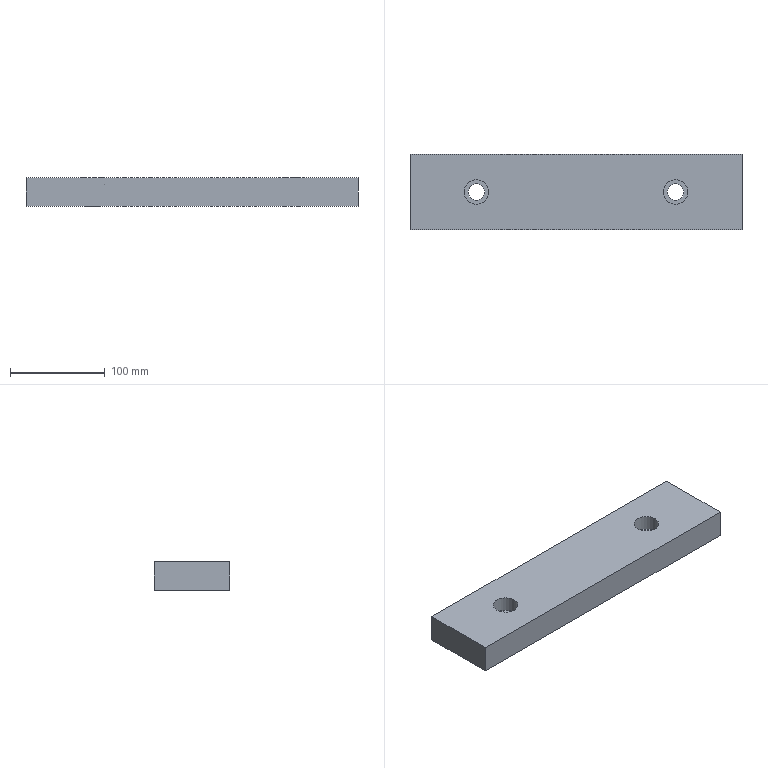Part | NX | features clamp plate 2 | 1 solid | 12 faces | box 350 x 80 x 30 mm | volume 816275 mm3 | plane 8 | cylinder 4 | commonest cylinder face diameters 17.5 x2 26 x2
STEP:
#1=CARTESIAN_POINT('',(-92.,0.,30.));
#2=VERTEX_POINT('',#1);
#3=CARTESIAN_POINT('',(-105.,0.,30.));
#4=DIRECTION('',(0.,0.,1.));
#5=DIRECTION('',(1.,0.,0.));
#6=AXIS2_PLACEMENT_3D('',#3,#4,#5);
#7=CIRCLE('',#6,13.);
#8=EDGE_CURVE('',#2,#2,#7,.F.);
#9=ORIENTED_EDGE('',*,*,#8,.F.);
#10=EDGE_LOOP('',(#9));
#11=FACE_BOUND('',#10,.T.);
#12=CARTESIAN_POINT('',(-92.,0.,14.));
#13=VERTEX_POINT('',#12);
#14=CARTESIAN_POINT('',(-105.,0.,14.));
#15=DIRECTION('',(0.,0.,1.));
#16=DIRECTION('',(1.,0.,0.));
#17=AXIS2_PLACEMENT_3D('',#14,#15,#16);
#18=CIRCLE('',#17,13.);
#19=EDGE_CURVE('',#13,#13,#18,.F.);
#20=ORIENTED_EDGE('',*,*,#19,.T.);
#21=EDGE_LOOP('',(#20));
#22=FACE_BOUND('',#21,.T.);
#23=CARTESIAN_POINT('',(-105.,0.,30.));
#24=DIRECTION('',(0.,0.,1.));
#25=DIRECTION('',(1.,0.,0.));
#26=AXIS2_PLACEMENT_3D('',#23,#24,#25);
#27=CYLINDRICAL_SURFACE('',#26,13.);
#28=ADVANCED_FACE('',(#11,#22),#27,.F.);
#29=CARTESIAN_POINT('',(118.,0.,30.));
#30=VERTEX_POINT('',#29);
#31=CARTESIAN_POINT('',(105.,0.,30.));
#32=DIRECTION('',(0.,0.,1.));
#33=DIRECTION('',(1.,0.,0.));
#34=AXIS2_PLACEMENT_3D('',#31,#32,#33);
#35=CIRCLE('',#34,13.);
#36=EDGE_CURVE('',#30,#30,#35,.F.);
#37=ORIENTED_EDGE('',*,*,#36,.F.);
#38=EDGE_LOOP('',(#37));
#39=FACE_BOUND('',#38,.T.);
#40=CARTESIAN_POINT('',(118.,0.,14.));
#41=VERTEX_POINT('',#40);
#42=CARTESIAN_POINT('',(105.,0.,14.));
#43=DIRECTION('',(0.,0.,1.));
#44=DIRECTION('',(1.,0.,0.));
#45=AXIS2_PLACEMENT_3D('',#42,#43,#44);
#46=CIRCLE('',#45,13.);
#47=EDGE_CURVE('',#41,#41,#46,.F.);
#48=ORIENTED_EDGE('',*,*,#47,.T.);
#49=EDGE_LOOP('',(#48));
#50=FACE_BOUND('',#49,.T.);
#51=CARTESIAN_POINT('',(105.,0.,30.));
#52=DIRECTION('',(0.,0.,1.));
#53=DIRECTION('',(1.,0.,0.));
#54=AXIS2_PLACEMENT_3D('',#51,#52,#53);
#55=CYLINDRICAL_SURFACE('',#54,13.);
#56=ADVANCED_FACE('',(#39,#50),#55,.F.);
#57=ORIENTED_EDGE('',*,*,#19,.F.);
#58=EDGE_LOOP('',(#57));
#59=FACE_BOUND('',#58,.T.);
#60=CARTESIAN_POINT('',(-96.25,0.,14.));
#61=VERTEX_POINT('',#60);
#62=CARTESIAN_POINT('',(-105.,0.,14.));
#63=DIRECTION('',(0.,0.,1.));
#64=DIRECTION('',(1.,0.,0.));
#65=AXIS2_PLACEMENT_3D('',#62,#63,#64);
#66=CIRCLE('',#65,8.75);
#67=EDGE_CURVE('',#61,#61,#66,.F.);
#68=ORIENTED_EDGE('',*,*,#67,.T.);
#69=EDGE_LOOP('',(#68));
#70=FACE_BOUND('',#69,.T.);
#71=CARTESIAN_POINT('',(-96.25,0.,14.));
#72=DIRECTION('',(0.,0.,-1.));
#73=DIRECTION('',(-1.,0.,0.));
#74=AXIS2_PLACEMENT_3D('',#71,#72,#73);
#75=PLANE('',#74);
#76=ADVANCED_FACE('',(#59,#70),#75,.F.);
#77=ORIENTED_EDGE('',*,*,#47,.F.);
#78=EDGE_LOOP('',(#77));
#79=FACE_BOUND('',#78,.T.);
#80=CARTESIAN_POINT('',(113.75,0.,14.));
#81=VERTEX_POINT('',#80);
#82=CARTESIAN_POINT('',(105.,0.,14.));
#83=DIRECTION('',(0.,0.,1.));
#84=DIRECTION('',(1.,0.,0.));
#85=AXIS2_PLACEMENT_3D('',#82,#83,#84);
#86=CIRCLE('',#85,8.75);
#87=EDGE_CURVE('',#81,#81,#86,.F.);
#88=ORIENTED_EDGE('',*,*,#87,.T.);
#89=EDGE_LOOP('',(#88));
#90=FACE_BOUND('',#89,.T.);
#91=CARTESIAN_POINT('',(113.75,0.,14.));
#92=DIRECTION('',(0.,0.,-1.));
#93=DIRECTION('',(-1.,0.,0.));
#94=AXIS2_PLACEMENT_3D('',#91,#92,#93);
#95=PLANE('',#94);
#96=ADVANCED_FACE('',(#79,#90),#95,.F.);
#97=CARTESIAN_POINT('',(-175.,40.,30.));
#98=VERTEX_POINT('',#97);
#99=CARTESIAN_POINT('',(-175.,-40.,30.));
#100=VERTEX_POINT('',#99);
#101=CARTESIAN_POINT('',(-175.,40.,30.));
#102=DIRECTION('',(0.,1.,0.));
#103=VECTOR('',#102,1000.);
#104=LINE('',#101,#103);
#105=EDGE_CURVE('',#98,#100,#104,.F.);
#106=ORIENTED_EDGE('',*,*,#105,.T.);
#107=CARTESIAN_POINT('',(175.,-40.,30.));
#108=VERTEX_POINT('',#107);
#109=CARTESIAN_POINT('',(-175.,-40.,30.));
#110=DIRECTION('',(1.,0.,0.));
#111=VECTOR('',#110,1000.);
#112=LINE('',#109,#111);
#113=EDGE_CURVE('',#100,#108,#112,.T.);
#114=ORIENTED_EDGE('',*,*,#113,.T.);
#115=CARTESIAN_POINT('',(175.,40.,30.));
#116=VERTEX_POINT('',#115);
#117=CARTESIAN_POINT('',(175.,40.,30.));
#118=DIRECTION('',(0.,1.,0.));
#119=VECTOR('',#118,1000.);
#120=LINE('',#117,#119);
#121=EDGE_CURVE('',#108,#116,#120,.T.);
#122=ORIENTED_EDGE('',*,*,#121,.T.);
#123=CARTESIAN_POINT('',(-175.,40.,30.));
#124=DIRECTION('',(1.,0.,0.));
#125=VECTOR('',#124,1000.);
#126=LINE('',#123,#125);
#127=EDGE_CURVE('',#116,#98,#126,.F.);
#128=ORIENTED_EDGE('',*,*,#127,.T.);
#129=EDGE_LOOP('',(#106,#114,#122,#128));
#130=FACE_BOUND('',#129,.T.);
#131=ORIENTED_EDGE('',*,*,#36,.T.);
#132=EDGE_LOOP('',(#131));
#133=FACE_BOUND('',#132,.T.);
#134=ORIENTED_EDGE('',*,*,#8,.T.);
#135=EDGE_LOOP('',(#134));
#136=FACE_BOUND('',#135,.T.);
#137=CARTESIAN_POINT('',(175.,-40.,30.));
#138=DIRECTION('',(0.,0.,1.));
#139=DIRECTION('',(1.,0.,0.));
#140=AXIS2_PLACEMENT_3D('',#137,#138,#139);
#141=PLANE('',#140);
#142=ADVANCED_FACE('',(#130,#133,#136),#141,.T.);
#143=CARTESIAN_POINT('',(-96.25,0.,0.));
#144=VERTEX_POINT('',#143);
#145=CARTESIAN_POINT('',(-105.,0.,0.));
#146=DIRECTION('',(0.,0.,1.));
#147=DIRECTION('',(1.,0.,0.));
#148=AXIS2_PLACEMENT_3D('',#145,#146,#147);
#149=CIRCLE('',#148,8.75);
#150=EDGE_CURVE('',#144,#144,#149,.F.);
#151=ORIENTED_EDGE('',*,*,#150,.T.);
#152=EDGE_LOOP('',(#151));
#153=FACE_BOUND('',#152,.T.);
#154=ORIENTED_EDGE('',*,*,#67,.F.);
#155=EDGE_LOOP('',(#154));
#156=FACE_BOUND('',#155,.T.);
#157=CARTESIAN_POINT('',(-105.,0.,30.));
#158=DIRECTION('',(0.,0.,1.));
#159=DIRECTION('',(1.,0.,0.));
#160=AXIS2_PLACEMENT_3D('',#157,#158,#159);
#161=CYLINDRICAL_SURFACE('',#160,8.75);
#162=ADVANCED_FACE('',(#153,#156),#161,.F.);
#163=CARTESIAN_POINT('',(113.75,0.,0.));
#164=VERTEX_POINT('',#163);
#165=CARTESIAN_POINT('',(105.,0.,0.));
#166=DIRECTION('',(0.,0.,1.));
#167=DIRECTION('',(1.,0.,0.));
#168=AXIS2_PLACEMENT_3D('',#165,#166,#167);
#169=CIRCLE('',#168,8.75);
#170=EDGE_CURVE('',#164,#164,#169,.F.);
#171=ORIENTED_EDGE('',*,*,#170,.T.);
#172=EDGE_LOOP('',(#171));
#173=FACE_BOUND('',#172,.T.);
#174=ORIENTED_EDGE('',*,*,#87,.F.);
#175=EDGE_LOOP('',(#174));
#176=FACE_BOUND('',#175,.T.);
#177=CARTESIAN_POINT('',(105.,0.,30.));
#178=DIRECTION('',(0.,0.,1.));
#179=DIRECTION('',(1.,0.,0.));
#180=AXIS2_PLACEMENT_3D('',#177,#178,#179);
#181=CYLINDRICAL_SURFACE('',#180,8.75);
#182=ADVANCED_FACE('',(#173,#176),#181,.F.);
#183=CARTESIAN_POINT('',(-175.,40.,0.));
#184=VERTEX_POINT('',#183);
#185=CARTESIAN_POINT('',(-175.,40.,30.));
#186=DIRECTION('',(0.,0.,-1.));
#187=VECTOR('',#186,1000.);
#188=LINE('',#185,#187);
#189=EDGE_CURVE('',#184,#98,#188,.F.);
#190=ORIENTED_EDGE('',*,*,#189,.T.);
#191=ORIENTED_EDGE('',*,*,#127,.F.);
#192=CARTESIAN_POINT('',(175.,40.,0.));
#193=VERTEX_POINT('',#192);
#194=CARTESIAN_POINT('',(175.,40.,30.));
#195=DIRECTION('',(0.,0.,1.));
#196=VECTOR('',#195,1000.);
#197=LINE('',#194,#196);
#198=EDGE_CURVE('',#116,#193,#197,.F.);
#199=ORIENTED_EDGE('',*,*,#198,.T.);
#200=CARTESIAN_POINT('',(175.,40.,0.));
#201=DIRECTION('',(1.,0.,0.));
#202=VECTOR('',#201,1000.);
#203=LINE('',#200,#202);
#204=EDGE_CURVE('',#193,#184,#203,.F.);
#205=ORIENTED_EDGE('',*,*,#204,.T.);
#206=EDGE_LOOP('',(#190,#191,#199,#205));
#207=FACE_BOUND('',#206,.T.);
#208=CARTESIAN_POINT('',(-175.,40.,30.));
#209=DIRECTION('',(0.,-1.,0.));
#210=DIRECTION('',(0.,0.,-1.));
#211=AXIS2_PLACEMENT_3D('',#208,#209,#210);
#212=PLANE('',#211);
#213=ADVANCED_FACE('',(#207),#212,.F.);
#214=CARTESIAN_POINT('',(-175.,-40.,0.));
#215=VERTEX_POINT('',#214);
#216=CARTESIAN_POINT('',(-175.,-40.,30.));
#217=DIRECTION('',(0.,0.,1.));
#218=VECTOR('',#217,1000.);
#219=LINE('',#216,#218);
#220=EDGE_CURVE('',#215,#100,#219,.T.);
#221=ORIENTED_EDGE('',*,*,#220,.T.);
#222=ORIENTED_EDGE('',*,*,#105,.F.);
#223=ORIENTED_EDGE('',*,*,#189,.F.);
#224=CARTESIAN_POINT('',(-175.,-40.,0.));
#225=DIRECTION('',(0.,1.,0.));
#226=VECTOR('',#225,1000.);
#227=LINE('',#224,#226);
#228=EDGE_CURVE('',#184,#215,#227,.F.);
#229=ORIENTED_EDGE('',*,*,#228,.T.);
#230=EDGE_LOOP('',(#221,#222,#223,#229));
#231=FACE_BOUND('',#230,.T.);
#232=CARTESIAN_POINT('',(-175.,40.,30.));
#233=DIRECTION('',(1.,0.,0.));
#234=DIRECTION('',(0.,0.,-1.));
#235=AXIS2_PLACEMENT_3D('',#232,#233,#234);
#236=PLANE('',#235);
#237=ADVANCED_FACE('',(#231),#236,.F.);
#238=CARTESIAN_POINT('',(175.,-40.,0.));
#239=VERTEX_POINT('',#238);
#240=CARTESIAN_POINT('',(175.,-40.,30.));
#241=DIRECTION('',(0.,0.,1.));
#242=VECTOR('',#241,1000.);
#243=LINE('',#240,#242);
#244=EDGE_CURVE('',#239,#108,#243,.T.);
#245=ORIENTED_EDGE('',*,*,#244,.T.);
#246=ORIENTED_EDGE('',*,*,#113,.F.);
#247=ORIENTED_EDGE('',*,*,#220,.F.);
#248=CARTESIAN_POINT('',(175.,-40.,0.));
#249=DIRECTION('',(1.,0.,0.));
#250=VECTOR('',#249,1000.);
#251=LINE('',#248,#250);
#252=EDGE_CURVE('',#215,#239,#251,.T.);
#253=ORIENTED_EDGE('',*,*,#252,.T.);
#254=EDGE_LOOP('',(#245,#246,#247,#253));
#255=FACE_BOUND('',#254,.T.);
#256=CARTESIAN_POINT('',(-175.,-40.,30.));
#257=DIRECTION('',(0.,1.,0.));
#258=DIRECTION('',(0.,0.,1.));
#259=AXIS2_PLACEMENT_3D('',#256,#257,#258);
#260=PLANE('',#259);
#261=ADVANCED_FACE('',(#255),#260,.F.);
#262=ORIENTED_EDGE('',*,*,#198,.F.);
#263=ORIENTED_EDGE('',*,*,#121,.F.);
#264=ORIENTED_EDGE('',*,*,#244,.F.);
#265=CARTESIAN_POINT('',(175.,-40.,0.));
#266=DIRECTION('',(0.,1.,0.));
#267=VECTOR('',#266,1000.);
#268=LINE('',#265,#267);
#269=EDGE_CURVE('',#239,#193,#268,.T.);
#270=ORIENTED_EDGE('',*,*,#269,.T.);
#271=EDGE_LOOP('',(#262,#263,#264,#270));
#272=FACE_BOUND('',#271,.T.);
#273=CARTESIAN_POINT('',(175.,40.,30.));
#274=DIRECTION('',(-1.,0.,0.));
#275=DIRECTION('',(0.,0.,1.));
#276=AXIS2_PLACEMENT_3D('',#273,#274,#275);
#277=PLANE('',#276);
#278=ADVANCED_FACE('',(#272),#277,.F.);
#279=ORIENTED_EDGE('',*,*,#252,.F.);
#280=ORIENTED_EDGE('',*,*,#228,.F.);
#281=ORIENTED_EDGE('',*,*,#204,.F.);
#282=ORIENTED_EDGE('',*,*,#269,.F.);
#283=EDGE_LOOP('',(#279,#280,#281,#282));
#284=FACE_BOUND('',#283,.T.);
#285=ORIENTED_EDGE('',*,*,#170,.F.);
#286=EDGE_LOOP('',(#285));
#287=FACE_BOUND('',#286,.T.);
#288=ORIENTED_EDGE('',*,*,#150,.F.);
#289=EDGE_LOOP('',(#288));
#290=FACE_BOUND('',#289,.T.);
#291=CARTESIAN_POINT('',(175.,-40.,0.));
#292=DIRECTION('',(0.,0.,1.));
#293=DIRECTION('',(1.,0.,0.));
#294=AXIS2_PLACEMENT_3D('',#291,#292,#293);
#295=PLANE('',#294);
#296=ADVANCED_FACE('',(#284,#287,#290),#295,.F.);
#297=CLOSED_SHELL('',(#28,#56,#76,#96,#142,#162,#182,#213,#237,#261,#278,#296));
#298=MANIFOLD_SOLID_BREP('',#297);
#299=(LENGTH_UNIT()NAMED_UNIT(*)SI_UNIT(.MILLI.,.METRE.));
#300=UNCERTAINTY_MEASURE_WITH_UNIT(LENGTH_MEASURE(0.00001),#299,'','');
#301=(NAMED_UNIT(*)PLANE_ANGLE_UNIT()SI_UNIT($,.RADIAN.));
#302=(NAMED_UNIT(*)SI_UNIT($,.STERADIAN.)SOLID_ANGLE_UNIT());
#303=(GEOMETRIC_REPRESENTATION_CONTEXT(3)GLOBAL_UNCERTAINTY_ASSIGNED_CONTEXT((#300))GLOBAL_UNIT_ASSIGNED_CONTEXT((#299,#301,#302))REPRESENTATION_CONTEXT('',''));
#304=ADVANCED_BREP_SHAPE_REPRESENTATION('',(#298),#303);